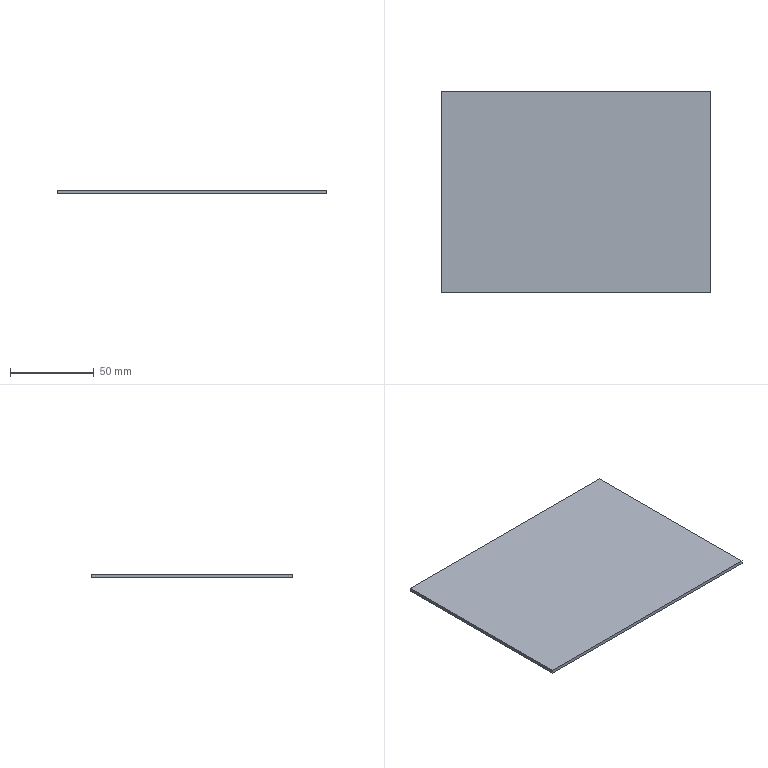Part | SolidWorks | features ICE 5, SheetMetal 2, SolidToSheetMetal 2, DeleteBody 1, Extrusion 1, FlatPattern 1, Shell 1 | 1 solid | 6 faces | box 160 x 120 x 2 mm | volume 38400 mm3 | plane 6
STEP:
#1=CARTESIAN_POINT('',(-340.,380.,-298.));
#2=VERTEX_POINT('',#1);
#3=CARTESIAN_POINT('',(-340.,380.,-300.));
#4=VERTEX_POINT('',#3);
#5=CARTESIAN_POINT('',(-340.,380.,-300.));
#6=DIRECTION('',(0.,0.,-1.));
#7=VECTOR('',#6,1000.);
#8=LINE('',#5,#7);
#9=EDGE_CURVE('',#2,#4,#8,.T.);
#10=ORIENTED_EDGE('',*,*,#9,.F.);
#11=CARTESIAN_POINT('',(-340.,260.,-298.));
#12=VERTEX_POINT('',#11);
#13=CARTESIAN_POINT('',(-340.,0.,-298.));
#14=DIRECTION('',(0.,-1.,0.));
#15=VECTOR('',#14,1000.);
#16=LINE('',#13,#15);
#17=EDGE_CURVE('',#2,#12,#16,.T.);
#18=ORIENTED_EDGE('',*,*,#17,.T.);
#19=CARTESIAN_POINT('',(-340.,260.,-300.));
#20=VERTEX_POINT('',#19);
#21=CARTESIAN_POINT('',(-340.,260.,-300.));
#22=DIRECTION('',(0.,0.,-1.));
#23=VECTOR('',#22,1000.);
#24=LINE('',#21,#23);
#25=EDGE_CURVE('',#12,#20,#24,.T.);
#26=ORIENTED_EDGE('',*,*,#25,.T.);
#27=CARTESIAN_POINT('',(-340.,380.,-300.));
#28=DIRECTION('',(0.,-1.,0.));
#29=VECTOR('',#28,1000.);
#30=LINE('',#27,#29);
#31=EDGE_CURVE('',#4,#20,#30,.T.);
#32=ORIENTED_EDGE('',*,*,#31,.F.);
#33=EDGE_LOOP('',(#10,#18,#26,#32));
#34=FACE_OUTER_BOUND('',#33,.T.);
#35=CARTESIAN_POINT('',(-340.,380.,-300.));
#36=DIRECTION('',(-1.,0.,0.));
#37=DIRECTION('',(0.,-1.,0.));
#38=AXIS2_PLACEMENT_3D('',#35,#36,#37);
#39=PLANE('',#38);
#40=ADVANCED_FACE('',(#34),#39,.F.);
#41=ORIENTED_EDGE('',*,*,#25,.F.);
#42=CARTESIAN_POINT('',(-500.,260.,-298.));
#43=VERTEX_POINT('',#42);
#44=CARTESIAN_POINT('',(0.,260.,-298.));
#45=DIRECTION('',(-1.,0.,0.));
#46=VECTOR('',#45,1000.);
#47=LINE('',#44,#46);
#48=EDGE_CURVE('',#12,#43,#47,.T.);
#49=ORIENTED_EDGE('',*,*,#48,.T.);
#50=CARTESIAN_POINT('',(-500.,260.,-300.));
#51=VERTEX_POINT('',#50);
#52=CARTESIAN_POINT('',(-500.,260.,-300.));
#53=DIRECTION('',(0.,0.,-1.));
#54=VECTOR('',#53,1000.);
#55=LINE('',#52,#54);
#56=EDGE_CURVE('',#43,#51,#55,.T.);
#57=ORIENTED_EDGE('',*,*,#56,.T.);
#58=CARTESIAN_POINT('',(-500.,260.,-300.));
#59=DIRECTION('',(-1.,0.,0.));
#60=VECTOR('',#59,1000.);
#61=LINE('',#58,#60);
#62=EDGE_CURVE('',#20,#51,#61,.T.);
#63=ORIENTED_EDGE('',*,*,#62,.F.);
#64=EDGE_LOOP('',(#41,#49,#57,#63));
#65=FACE_OUTER_BOUND('',#64,.T.);
#66=CARTESIAN_POINT('',(-500.,260.,-300.));
#67=DIRECTION('',(0.,1.,0.));
#68=DIRECTION('',(-1.,0.,0.));
#69=AXIS2_PLACEMENT_3D('',#66,#67,#68);
#70=PLANE('',#69);
#71=ADVANCED_FACE('',(#65),#70,.F.);
#72=ORIENTED_EDGE('',*,*,#56,.F.);
#73=CARTESIAN_POINT('',(-500.,380.,-298.));
#74=VERTEX_POINT('',#73);
#75=CARTESIAN_POINT('',(-500.,0.,-298.));
#76=DIRECTION('',(0.,1.,0.));
#77=VECTOR('',#76,1000.);
#78=LINE('',#75,#77);
#79=EDGE_CURVE('',#43,#74,#78,.T.);
#80=ORIENTED_EDGE('',*,*,#79,.T.);
#81=CARTESIAN_POINT('',(-500.,380.,-300.));
#82=VERTEX_POINT('',#81);
#83=CARTESIAN_POINT('',(-500.,380.,-300.));
#84=DIRECTION('',(0.,0.,-1.));
#85=VECTOR('',#84,1000.);
#86=LINE('',#83,#85);
#87=EDGE_CURVE('',#74,#82,#86,.T.);
#88=ORIENTED_EDGE('',*,*,#87,.T.);
#89=CARTESIAN_POINT('',(-500.,380.,-300.));
#90=DIRECTION('',(0.,1.,0.));
#91=VECTOR('',#90,1000.);
#92=LINE('',#89,#91);
#93=EDGE_CURVE('',#51,#82,#92,.T.);
#94=ORIENTED_EDGE('',*,*,#93,.F.);
#95=EDGE_LOOP('',(#72,#80,#88,#94));
#96=FACE_OUTER_BOUND('',#95,.T.);
#97=CARTESIAN_POINT('',(-500.,380.,-300.));
#98=DIRECTION('',(1.,0.,0.));
#99=DIRECTION('',(0.,1.,0.));
#100=AXIS2_PLACEMENT_3D('',#97,#98,#99);
#101=PLANE('',#100);
#102=ADVANCED_FACE('',(#96),#101,.F.);
#103=CARTESIAN_POINT('',(0.,380.,-298.));
#104=DIRECTION('',(1.,0.,0.));
#105=VECTOR('',#104,1000.);
#106=LINE('',#103,#105);
#107=EDGE_CURVE('',#74,#2,#106,.T.);
#108=ORIENTED_EDGE('',*,*,#107,.T.);
#109=ORIENTED_EDGE('',*,*,#9,.T.);
#110=CARTESIAN_POINT('',(-500.,380.,-300.));
#111=DIRECTION('',(1.,0.,0.));
#112=VECTOR('',#111,1000.);
#113=LINE('',#110,#112);
#114=EDGE_CURVE('',#82,#4,#113,.T.);
#115=ORIENTED_EDGE('',*,*,#114,.F.);
#116=ORIENTED_EDGE('',*,*,#87,.F.);
#117=EDGE_LOOP('',(#108,#109,#115,#116));
#118=FACE_OUTER_BOUND('',#117,.T.);
#119=CARTESIAN_POINT('',(-500.,380.,-300.));
#120=DIRECTION('',(0.,-1.,0.));
#121=DIRECTION('',(1.,0.,0.));
#122=AXIS2_PLACEMENT_3D('',#119,#120,#121);
#123=PLANE('',#122);
#124=ADVANCED_FACE('',(#118),#123,.F.);
#125=ORIENTED_EDGE('',*,*,#93,.T.);
#126=ORIENTED_EDGE('',*,*,#114,.T.);
#127=ORIENTED_EDGE('',*,*,#31,.T.);
#128=ORIENTED_EDGE('',*,*,#62,.T.);
#129=EDGE_LOOP('',(#125,#126,#127,#128));
#130=FACE_OUTER_BOUND('',#129,.T.);
#131=CARTESIAN_POINT('',(0.,0.,-300.));
#132=DIRECTION('',(0.,0.,1.));
#133=DIRECTION('',(1.,0.,0.));
#134=AXIS2_PLACEMENT_3D('',#131,#132,#133);
#135=PLANE('',#134);
#136=ADVANCED_FACE('',(#130),#135,.F.);
#137=ORIENTED_EDGE('',*,*,#79,.F.);
#138=ORIENTED_EDGE('',*,*,#48,.F.);
#139=ORIENTED_EDGE('',*,*,#17,.F.);
#140=ORIENTED_EDGE('',*,*,#107,.F.);
#141=EDGE_LOOP('',(#137,#138,#139,#140));
#142=FACE_OUTER_BOUND('',#141,.T.);
#143=CARTESIAN_POINT('',(0.,0.,-298.));
#144=DIRECTION('',(0.,0.,1.));
#145=DIRECTION('',(1.,0.,0.));
#146=AXIS2_PLACEMENT_3D('',#143,#144,#145);
#147=PLANE('',#146);
#148=ADVANCED_FACE('',(#142),#147,.T.);
#149=CLOSED_SHELL('',(#40,#71,#102,#124,#136,#148));
#150=MANIFOLD_SOLID_BREP('',#149);
#151=CARTESIAN_POINT('',(0.,0.,0.));
#152=DIRECTION('',(0.,0.,1.));
#153=DIRECTION('',(1.,0.,0.));
#154=AXIS2_PLACEMENT_3D('',#151,#152,#153);
#155=(LENGTH_UNIT()NAMED_UNIT(*)SI_UNIT(.MILLI.,.METRE.));
#156=UNCERTAINTY_MEASURE_WITH_UNIT(LENGTH_MEASURE(0.00001),#155,'','');
#157=(NAMED_UNIT(*)PLANE_ANGLE_UNIT()SI_UNIT($,.RADIAN.));
#158=(NAMED_UNIT(*)SI_UNIT($,.STERADIAN.)SOLID_ANGLE_UNIT());
#159=(GEOMETRIC_REPRESENTATION_CONTEXT(3)GLOBAL_UNCERTAINTY_ASSIGNED_CONTEXT((#156))GLOBAL_UNIT_ASSIGNED_CONTEXT((#155,#157,#158))REPRESENTATION_CONTEXT('',''));
#160=ADVANCED_BREP_SHAPE_REPRESENTATION('',(#150,#154),#159);